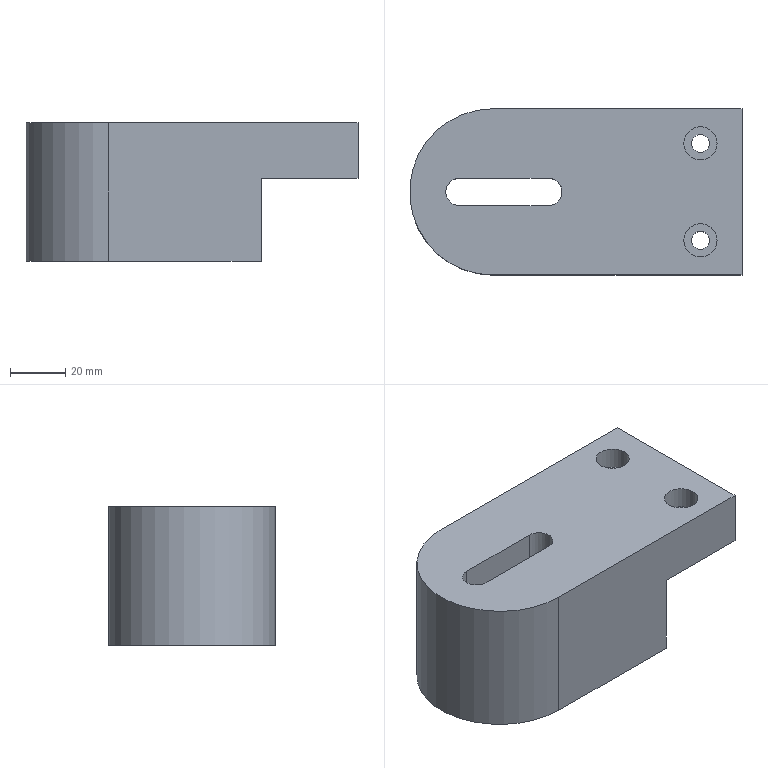Part | NX | 1 solid | 21 faces | box 120 x 60 x 50 mm | volume 252472 mm3 | plane 12 | cylinder 9 | commonest cylinder face diameters 12 x3 6.5 x2 10 x2 5 x1 60 x1
STEP:
#1=CARTESIAN_POINT('',(25.,-30.,-25.));
#2=VERTEX_POINT('',#1);
#3=CARTESIAN_POINT('',(25.,30.,-25.));
#4=VERTEX_POINT('',#3);
#5=CARTESIAN_POINT('',(25.,-30.,-25.));
#6=DIRECTION('',(0.,1.,0.));
#7=VECTOR('',#6,1.);
#8=LINE('',#5,#7);
#9=EDGE_CURVE('',#2,#4,#8,.T.);
#10=ORIENTED_EDGE('',*,*,#9,.F.);
#11=CARTESIAN_POINT('',(-30.,-30.,-25.));
#12=VERTEX_POINT('',#11);
#13=CARTESIAN_POINT('',(-30.,-30.,-25.));
#14=DIRECTION('',(1.,0.,0.));
#15=VECTOR('',#14,1.);
#16=LINE('',#13,#15);
#17=EDGE_CURVE('',#12,#2,#16,.T.);
#18=ORIENTED_EDGE('',*,*,#17,.F.);
#19=CARTESIAN_POINT('',(-30.,30.,-25.));
#20=VERTEX_POINT('',#19);
#21=CARTESIAN_POINT('',(-30.,0.,-25.));
#22=DIRECTION('',(0.,0.,1.));
#23=DIRECTION('',(0.,1.,0.));
#24=AXIS2_PLACEMENT_3D('',#21,#22,#23);
#25=CIRCLE('',#24,30.);
#26=EDGE_CURVE('',#20,#12,#25,.T.);
#27=ORIENTED_EDGE('',*,*,#26,.F.);
#28=CARTESIAN_POINT('',(25.,30.,-25.));
#29=DIRECTION('',(-1.,0.,0.));
#30=VECTOR('',#29,1.);
#31=LINE('',#28,#30);
#32=EDGE_CURVE('',#4,#20,#31,.T.);
#33=ORIENTED_EDGE('',*,*,#32,.F.);
#34=EDGE_LOOP('',(#10,#18,#27,#33));
#35=FACE_BOUND('',#34,.T.);
#36=CARTESIAN_POINT('',(-42.,5.,-25.));
#37=VERTEX_POINT('',#36);
#38=CARTESIAN_POINT('',(-42.,-5.,-25.));
#39=VERTEX_POINT('',#38);
#40=CARTESIAN_POINT('',(-42.,0.,-25.));
#41=DIRECTION('',(0.,0.,1.));
#42=DIRECTION('',(0.,1.,0.));
#43=AXIS2_PLACEMENT_3D('',#40,#41,#42);
#44=CIRCLE('',#43,5.);
#45=EDGE_CURVE('',#37,#39,#44,.T.);
#46=ORIENTED_EDGE('',*,*,#45,.T.);
#47=CARTESIAN_POINT('',(-10.,-5.,-25.));
#48=VERTEX_POINT('',#47);
#49=CARTESIAN_POINT('',(-42.,-5.,-25.));
#50=DIRECTION('',(1.,0.,0.));
#51=VECTOR('',#50,1.);
#52=LINE('',#49,#51);
#53=EDGE_CURVE('',#39,#48,#52,.T.);
#54=ORIENTED_EDGE('',*,*,#53,.T.);
#55=CARTESIAN_POINT('',(-10.,5.,-25.));
#56=VERTEX_POINT('',#55);
#57=CARTESIAN_POINT('',(-10.,0.,-25.));
#58=DIRECTION('',(0.,0.,1.));
#59=DIRECTION('',(0.,-1.,0.));
#60=AXIS2_PLACEMENT_3D('',#57,#58,#59);
#61=CIRCLE('',#60,5.);
#62=EDGE_CURVE('',#48,#56,#61,.T.);
#63=ORIENTED_EDGE('',*,*,#62,.T.);
#64=CARTESIAN_POINT('',(-10.,5.,-25.));
#65=DIRECTION('',(-1.,0.,0.));
#66=VECTOR('',#65,1.);
#67=LINE('',#64,#66);
#68=EDGE_CURVE('',#56,#37,#67,.T.);
#69=ORIENTED_EDGE('',*,*,#68,.T.);
#70=EDGE_LOOP('',(#46,#54,#63,#69));
#71=FACE_BOUND('',#70,.T.);
#72=CARTESIAN_POINT('',(0.,0.,-25.));
#73=DIRECTION('',(0.,0.,1.));
#74=DIRECTION('',(1.,0.,0.));
#75=AXIS2_PLACEMENT_3D('',#72,#73,#74);
#76=PLANE('',#75);
#77=ADVANCED_FACE('',(#35,#71),#76,.F.);
#78=CARTESIAN_POINT('',(-30.,-30.,25.));
#79=VERTEX_POINT('',#78);
#80=CARTESIAN_POINT('',(-30.,30.,25.));
#81=VERTEX_POINT('',#80);
#82=CARTESIAN_POINT('',(-30.,0.,25.));
#83=DIRECTION('',(0.,0.,-1.));
#84=DIRECTION('',(0.,-1.,0.));
#85=AXIS2_PLACEMENT_3D('',#82,#83,#84);
#86=CIRCLE('',#85,30.);
#87=EDGE_CURVE('',#79,#81,#86,.T.);
#88=ORIENTED_EDGE('',*,*,#87,.F.);
#89=CARTESIAN_POINT('',(60.,-30.,25.));
#90=VERTEX_POINT('',#89);
#91=CARTESIAN_POINT('',(-30.,-30.,25.));
#92=DIRECTION('',(1.,0.,0.));
#93=VECTOR('',#92,1.);
#94=LINE('',#91,#93);
#95=EDGE_CURVE('',#79,#90,#94,.T.);
#96=ORIENTED_EDGE('',*,*,#95,.T.);
#97=CARTESIAN_POINT('',(60.,30.,25.));
#98=VERTEX_POINT('',#97);
#99=CARTESIAN_POINT('',(60.,-30.,25.));
#100=DIRECTION('',(0.,1.,0.));
#101=VECTOR('',#100,1.);
#102=LINE('',#99,#101);
#103=EDGE_CURVE('',#90,#98,#102,.T.);
#104=ORIENTED_EDGE('',*,*,#103,.T.);
#105=CARTESIAN_POINT('',(60.,30.,25.));
#106=DIRECTION('',(-1.,0.,0.));
#107=VECTOR('',#106,1.);
#108=LINE('',#105,#107);
#109=EDGE_CURVE('',#98,#81,#108,.T.);
#110=ORIENTED_EDGE('',*,*,#109,.T.);
#111=EDGE_LOOP('',(#88,#96,#104,#110));
#112=FACE_BOUND('',#111,.T.);
#113=CARTESIAN_POINT('',(-42.,5.,25.));
#114=VERTEX_POINT('',#113);
#115=CARTESIAN_POINT('',(-42.,-5.,25.));
#116=VERTEX_POINT('',#115);
#117=CARTESIAN_POINT('',(-42.,0.,25.));
#118=DIRECTION('',(0.,0.,1.));
#119=DIRECTION('',(0.,1.,0.));
#120=AXIS2_PLACEMENT_3D('',#117,#118,#119);
#121=CIRCLE('',#120,5.);
#122=EDGE_CURVE('',#114,#116,#121,.T.);
#123=ORIENTED_EDGE('',*,*,#122,.F.);
#124=CARTESIAN_POINT('',(-10.,5.,25.));
#125=VERTEX_POINT('',#124);
#126=CARTESIAN_POINT('',(-10.,5.,25.));
#127=DIRECTION('',(-1.,0.,0.));
#128=VECTOR('',#127,1.);
#129=LINE('',#126,#128);
#130=EDGE_CURVE('',#125,#114,#129,.T.);
#131=ORIENTED_EDGE('',*,*,#130,.F.);
#132=CARTESIAN_POINT('',(-10.,-5.,25.));
#133=VERTEX_POINT('',#132);
#134=CARTESIAN_POINT('',(-10.,0.,25.));
#135=DIRECTION('',(0.,0.,1.));
#136=DIRECTION('',(0.,-1.,0.));
#137=AXIS2_PLACEMENT_3D('',#134,#135,#136);
#138=CIRCLE('',#137,5.);
#139=EDGE_CURVE('',#133,#125,#138,.T.);
#140=ORIENTED_EDGE('',*,*,#139,.F.);
#141=CARTESIAN_POINT('',(-42.,-5.,25.));
#142=DIRECTION('',(1.,0.,0.));
#143=VECTOR('',#142,1.);
#144=LINE('',#141,#143);
#145=EDGE_CURVE('',#116,#133,#144,.T.);
#146=ORIENTED_EDGE('',*,*,#145,.F.);
#147=EDGE_LOOP('',(#123,#131,#140,#146));
#148=FACE_BOUND('',#147,.T.);
#149=CARTESIAN_POINT('',(51.,17.5,25.));
#150=VERTEX_POINT('',#149);
#151=CARTESIAN_POINT('',(45.,17.5,25.));
#152=DIRECTION('',(0.,0.,1.));
#153=DIRECTION('',(1.,0.,0.));
#154=AXIS2_PLACEMENT_3D('',#151,#152,#153);
#155=CIRCLE('',#154,6.);
#156=EDGE_CURVE('',#150,#150,#155,.T.);
#157=ORIENTED_EDGE('',*,*,#156,.F.);
#158=EDGE_LOOP('',(#157));
#159=FACE_BOUND('',#158,.T.);
#160=CARTESIAN_POINT('',(51.,-17.5,25.));
#161=VERTEX_POINT('',#160);
#162=CARTESIAN_POINT('',(45.,-17.5,25.));
#163=DIRECTION('',(0.,0.,1.));
#164=DIRECTION('',(1.,0.,0.));
#165=AXIS2_PLACEMENT_3D('',#162,#163,#164);
#166=CIRCLE('',#165,6.);
#167=EDGE_CURVE('',#161,#161,#166,.T.);
#168=ORIENTED_EDGE('',*,*,#167,.F.);
#169=EDGE_LOOP('',(#168));
#170=FACE_BOUND('',#169,.T.);
#171=CARTESIAN_POINT('',(0.,0.,25.));
#172=DIRECTION('',(0.,0.,1.));
#173=DIRECTION('',(1.,0.,0.));
#174=AXIS2_PLACEMENT_3D('',#171,#172,#173);
#175=PLANE('',#174);
#176=ADVANCED_FACE('',(#112,#148,#159,#170),#175,.T.);
#177=CARTESIAN_POINT('',(60.,-30.,5.));
#178=VERTEX_POINT('',#177);
#179=CARTESIAN_POINT('',(25.,-30.,5.));
#180=VERTEX_POINT('',#179);
#181=CARTESIAN_POINT('',(60.,-30.,5.));
#182=DIRECTION('',(-1.,0.,0.));
#183=VECTOR('',#182,1.);
#184=LINE('',#181,#183);
#185=EDGE_CURVE('',#178,#180,#184,.T.);
#186=ORIENTED_EDGE('',*,*,#185,.F.);
#187=CARTESIAN_POINT('',(60.,-30.,5.));
#188=DIRECTION('',(0.,0.,1.));
#189=VECTOR('',#188,1.);
#190=LINE('',#187,#189);
#191=EDGE_CURVE('',#178,#90,#190,.T.);
#192=ORIENTED_EDGE('',*,*,#191,.T.);
#193=ORIENTED_EDGE('',*,*,#95,.F.);
#194=CARTESIAN_POINT('',(-30.,-30.,25.));
#195=DIRECTION('',(0.,0.,-1.));
#196=VECTOR('',#195,1.);
#197=LINE('',#194,#196);
#198=EDGE_CURVE('',#79,#12,#197,.T.);
#199=ORIENTED_EDGE('',*,*,#198,.T.);
#200=ORIENTED_EDGE('',*,*,#17,.T.);
#201=CARTESIAN_POINT('',(25.,-30.,-25.));
#202=DIRECTION('',(0.,0.,1.));
#203=VECTOR('',#202,1.);
#204=LINE('',#201,#203);
#205=EDGE_CURVE('',#2,#180,#204,.T.);
#206=ORIENTED_EDGE('',*,*,#205,.T.);
#207=EDGE_LOOP('',(#186,#192,#193,#199,#200,#206));
#208=FACE_OUTER_BOUND('',#207,.T.);
#209=CARTESIAN_POINT('',(-60.,-30.,-25.));
#210=DIRECTION('',(0.,-1.,0.));
#211=DIRECTION('',(0.,0.,-1.));
#212=AXIS2_PLACEMENT_3D('',#209,#210,#211);
#213=PLANE('',#212);
#214=ADVANCED_FACE('',(#208),#213,.T.);
#215=CARTESIAN_POINT('',(60.,30.,5.));
#216=VERTEX_POINT('',#215);
#217=CARTESIAN_POINT('',(60.,-30.,5.));
#218=DIRECTION('',(0.,1.,0.));
#219=VECTOR('',#218,1.);
#220=LINE('',#217,#219);
#221=EDGE_CURVE('',#178,#216,#220,.T.);
#222=ORIENTED_EDGE('',*,*,#221,.T.);
#223=CARTESIAN_POINT('',(60.,30.,5.));
#224=DIRECTION('',(0.,0.,1.));
#225=VECTOR('',#224,1.);
#226=LINE('',#223,#225);
#227=EDGE_CURVE('',#216,#98,#226,.T.);
#228=ORIENTED_EDGE('',*,*,#227,.T.);
#229=ORIENTED_EDGE('',*,*,#103,.F.);
#230=ORIENTED_EDGE('',*,*,#191,.F.);
#231=EDGE_LOOP('',(#222,#228,#229,#230));
#232=FACE_BOUND('',#231,.T.);
#233=CARTESIAN_POINT('',(60.,0.,9.));
#234=VERTEX_POINT('',#233);
#235=CARTESIAN_POINT('',(60.,0.,15.));
#236=DIRECTION('',(1.,0.,0.));
#237=DIRECTION('',(0.,0.,-1.));
#238=AXIS2_PLACEMENT_3D('',#235,#236,#237);
#239=CIRCLE('',#238,6.);
#240=EDGE_CURVE('',#234,#234,#239,.T.);
#241=ORIENTED_EDGE('',*,*,#240,.F.);
#242=EDGE_LOOP('',(#241));
#243=FACE_BOUND('',#242,.T.);
#244=CARTESIAN_POINT('',(60.,-30.,-25.));
#245=DIRECTION('',(1.,0.,0.));
#246=DIRECTION('',(0.,0.,-1.));
#247=AXIS2_PLACEMENT_3D('',#244,#245,#246);
#248=PLANE('',#247);
#249=ADVANCED_FACE('',(#232,#243),#248,.T.);
#250=CARTESIAN_POINT('',(25.,30.,5.));
#251=VERTEX_POINT('',#250);
#252=CARTESIAN_POINT('',(60.,30.,5.));
#253=DIRECTION('',(-1.,0.,0.));
#254=VECTOR('',#253,1.);
#255=LINE('',#252,#254);
#256=EDGE_CURVE('',#216,#251,#255,.T.);
#257=ORIENTED_EDGE('',*,*,#256,.T.);
#258=CARTESIAN_POINT('',(25.,30.,-25.));
#259=DIRECTION('',(0.,0.,1.));
#260=VECTOR('',#259,1.);
#261=LINE('',#258,#260);
#262=EDGE_CURVE('',#4,#251,#261,.T.);
#263=ORIENTED_EDGE('',*,*,#262,.F.);
#264=ORIENTED_EDGE('',*,*,#32,.T.);
#265=CARTESIAN_POINT('',(-30.,30.,25.));
#266=DIRECTION('',(0.,0.,-1.));
#267=VECTOR('',#266,1.);
#268=LINE('',#265,#267);
#269=EDGE_CURVE('',#81,#20,#268,.T.);
#270=ORIENTED_EDGE('',*,*,#269,.F.);
#271=ORIENTED_EDGE('',*,*,#109,.F.);
#272=ORIENTED_EDGE('',*,*,#227,.F.);
#273=EDGE_LOOP('',(#257,#263,#264,#270,#271,#272));
#274=FACE_OUTER_BOUND('',#273,.T.);
#275=CARTESIAN_POINT('',(60.,30.,-25.));
#276=DIRECTION('',(0.,1.,0.));
#277=DIRECTION('',(0.,0.,1.));
#278=AXIS2_PLACEMENT_3D('',#275,#276,#277);
#279=PLANE('',#278);
#280=ADVANCED_FACE('',(#274),#279,.T.);
#281=ORIENTED_EDGE('',*,*,#87,.T.);
#282=ORIENTED_EDGE('',*,*,#269,.T.);
#283=ORIENTED_EDGE('',*,*,#26,.T.);
#284=ORIENTED_EDGE('',*,*,#198,.F.);
#285=EDGE_LOOP('',(#281,#282,#283,#284));
#286=FACE_OUTER_BOUND('',#285,.T.);
#287=CARTESIAN_POINT('',(-30.,0.,25.231));
#288=DIRECTION('',(0.,0.,-1.));
#289=DIRECTION('',(-1.,0.,0.));
#290=AXIS2_PLACEMENT_3D('',#287,#288,#289);
#291=CYLINDRICAL_SURFACE('',#290,30.);
#292=ADVANCED_FACE('',(#286),#291,.T.);
#293=ORIENTED_EDGE('',*,*,#185,.T.);
#294=CARTESIAN_POINT('',(25.,-30.,5.));
#295=DIRECTION('',(0.,1.,0.));
#296=VECTOR('',#295,1.);
#297=LINE('',#294,#296);
#298=EDGE_CURVE('',#180,#251,#297,.T.);
#299=ORIENTED_EDGE('',*,*,#298,.T.);
#300=ORIENTED_EDGE('',*,*,#256,.F.);
#301=ORIENTED_EDGE('',*,*,#221,.F.);
#302=EDGE_LOOP('',(#293,#299,#300,#301));
#303=FACE_BOUND('',#302,.T.);
#304=CARTESIAN_POINT('',(48.25,17.5,5.));
#305=VERTEX_POINT('',#304);
#306=CARTESIAN_POINT('',(45.,17.5,5.));
#307=DIRECTION('',(0.,0.,1.));
#308=DIRECTION('',(1.,0.,0.));
#309=AXIS2_PLACEMENT_3D('',#306,#307,#308);
#310=CIRCLE('',#309,3.25);
#311=EDGE_CURVE('',#305,#305,#310,.T.);
#312=ORIENTED_EDGE('',*,*,#311,.T.);
#313=EDGE_LOOP('',(#312));
#314=FACE_BOUND('',#313,.T.);
#315=CARTESIAN_POINT('',(48.25,-17.5,5.));
#316=VERTEX_POINT('',#315);
#317=CARTESIAN_POINT('',(45.,-17.5,5.));
#318=DIRECTION('',(0.,0.,1.));
#319=DIRECTION('',(1.,0.,0.));
#320=AXIS2_PLACEMENT_3D('',#317,#318,#319);
#321=CIRCLE('',#320,3.25);
#322=EDGE_CURVE('',#316,#316,#321,.T.);
#323=ORIENTED_EDGE('',*,*,#322,.T.);
#324=EDGE_LOOP('',(#323));
#325=FACE_BOUND('',#324,.T.);
#326=CARTESIAN_POINT('',(0.,0.,5.));
#327=DIRECTION('',(0.,0.,-1.));
#328=DIRECTION('',(-1.,0.,0.));
#329=AXIS2_PLACEMENT_3D('',#326,#327,#328);
#330=PLANE('',#329);
#331=ADVANCED_FACE('',(#303,#314,#325),#330,.T.);
#332=ORIENTED_EDGE('',*,*,#9,.T.);
#333=ORIENTED_EDGE('',*,*,#262,.T.);
#334=ORIENTED_EDGE('',*,*,#298,.F.);
#335=ORIENTED_EDGE('',*,*,#205,.F.);
#336=EDGE_LOOP('',(#332,#333,#334,#335));
#337=FACE_OUTER_BOUND('',#336,.T.);
#338=CARTESIAN_POINT('',(25.,-30.,-25.));
#339=DIRECTION('',(-1.,0.,0.));
#340=DIRECTION('',(0.,0.,1.));
#341=AXIS2_PLACEMENT_3D('',#338,#339,#340);
#342=PLANE('',#341);
#343=ADVANCED_FACE('',(#337),#342,.F.);
#344=ORIENTED_EDGE('',*,*,#45,.F.);
#345=CARTESIAN_POINT('',(-42.,5.,25.));
#346=DIRECTION('',(0.,0.,-1.));
#347=VECTOR('',#346,1.);
#348=LINE('',#345,#347);
#349=EDGE_CURVE('',#114,#37,#348,.T.);
#350=ORIENTED_EDGE('',*,*,#349,.F.);
#351=ORIENTED_EDGE('',*,*,#122,.T.);
#352=CARTESIAN_POINT('',(-42.,-5.,25.));
#353=DIRECTION('',(0.,0.,-1.));
#354=VECTOR('',#353,1.);
#355=LINE('',#352,#354);
#356=EDGE_CURVE('',#116,#39,#355,.T.);
#357=ORIENTED_EDGE('',*,*,#356,.T.);
#358=EDGE_LOOP('',(#344,#350,#351,#357));
#359=FACE_OUTER_BOUND('',#358,.T.);
#360=CARTESIAN_POINT('',(-42.,0.,25.));
#361=DIRECTION('',(0.,0.,1.));
#362=DIRECTION('',(1.,0.,0.));
#363=AXIS2_PLACEMENT_3D('',#360,#361,#362);
#364=CYLINDRICAL_SURFACE('',#363,5.);
#365=ADVANCED_FACE('',(#359),#364,.F.);
#366=ORIENTED_EDGE('',*,*,#53,.F.);
#367=ORIENTED_EDGE('',*,*,#356,.F.);
#368=ORIENTED_EDGE('',*,*,#145,.T.);
#369=CARTESIAN_POINT('',(-10.,-5.,25.));
#370=DIRECTION('',(0.,0.,-1.));
#371=VECTOR('',#370,1.);
#372=LINE('',#369,#371);
#373=EDGE_CURVE('',#133,#48,#372,.T.);
#374=ORIENTED_EDGE('',*,*,#373,.T.);
#375=EDGE_LOOP('',(#366,#367,#368,#374));
#376=FACE_OUTER_BOUND('',#375,.T.);
#377=CARTESIAN_POINT('',(-42.,-5.,25.));
#378=DIRECTION('',(0.,-1.,0.));
#379=DIRECTION('',(0.,0.,-1.));
#380=AXIS2_PLACEMENT_3D('',#377,#378,#379);
#381=PLANE('',#380);
#382=ADVANCED_FACE('',(#376),#381,.F.);
#383=ORIENTED_EDGE('',*,*,#62,.F.);
#384=ORIENTED_EDGE('',*,*,#373,.F.);
#385=ORIENTED_EDGE('',*,*,#139,.T.);
#386=CARTESIAN_POINT('',(-10.,5.,25.));
#387=DIRECTION('',(0.,0.,-1.));
#388=VECTOR('',#387,1.);
#389=LINE('',#386,#388);
#390=EDGE_CURVE('',#125,#56,#389,.T.);
#391=ORIENTED_EDGE('',*,*,#390,.T.);
#392=EDGE_LOOP('',(#383,#384,#385,#391));
#393=FACE_BOUND('',#392,.T.);
#394=CARTESIAN_POINT('',(-5.,-0.000000402,12.5));
#395=VERTEX_POINT('',#394);
#396=CARTESIAN_POINT('',(-5.,-0.000000402,12.5));
#397=CARTESIAN_POINT('',(-5.,0.262,12.5));
#398=CARTESIAN_POINT('',(-5.022,0.5275,12.543));
#399=CARTESIAN_POINT('',(-5.06,0.7739,12.623));
#400=CARTESIAN_POINT('',(-5.099,1.02,12.703));
#401=CARTESIAN_POINT('',(-5.155,1.253,12.822));
#402=CARTESIAN_POINT('',(-5.218,1.459,12.97));
#403=CARTESIAN_POINT('',(-5.284,1.678,13.127));
#404=CARTESIAN_POINT('',(-5.36,1.871,13.321));
#405=CARTESIAN_POINT('',(-5.43,2.028,13.538));
#406=CARTESIAN_POINT('',(-5.505,2.197,13.773));
#407=CARTESIAN_POINT('',(-5.574,2.328,14.043));
#408=CARTESIAN_POINT('',(-5.618,2.408,14.327));
#409=CARTESIAN_POINT('',(-5.659,2.482,14.594));
#410=CARTESIAN_POINT('',(-5.677,2.513,14.883));
#411=CARTESIAN_POINT('',(-5.667,2.495,15.162));
#412=CARTESIAN_POINT('',(-5.658,2.479,15.408));
#413=CARTESIAN_POINT('',(-5.626,2.425,15.654));
#414=CARTESIAN_POINT('',(-5.581,2.34,15.881));
#415=CARTESIAN_POINT('',(-5.535,2.252,16.114));
#416=CARTESIAN_POINT('',(-5.473,2.129,16.333));
#417=CARTESIAN_POINT('',(-5.409,1.98,16.527));
#418=CARTESIAN_POINT('',(-5.336,1.811,16.745));
#419=CARTESIAN_POINT('',(-5.258,1.605,16.937));
#420=CARTESIAN_POINT('',(-5.192,1.373,17.089));
#421=CARTESIAN_POINT('',(-5.123,1.131,17.248));
#422=CARTESIAN_POINT('',(-5.065,0.8533,17.368));
#423=CARTESIAN_POINT('',(-5.032,0.5649,17.435));
#424=CARTESIAN_POINT('',(-5.002,0.3005,17.497));
#425=CARTESIAN_POINT('',(-4.993,0.01906,17.515));
#426=CARTESIAN_POINT('',(-5.006,-0.2523,17.487));
#427=CARTESIAN_POINT('',(-5.019,-0.5027,17.462));
#428=CARTESIAN_POINT('',(-5.051,-0.7513,17.397));
#429=CARTESIAN_POINT('',(-5.097,-0.9794,17.3));
#430=CARTESIAN_POINT('',(-5.144,-1.214,17.2));
#431=CARTESIAN_POINT('',(-5.206,-1.433,17.064));
#432=CARTESIAN_POINT('',(-5.271,-1.624,16.901));
#433=CARTESIAN_POINT('',(-5.343,-1.834,16.721));
#434=CARTESIAN_POINT('',(-5.421,-2.015,16.506));
#435=CARTESIAN_POINT('',(-5.488,-2.155,16.267));
#436=CARTESIAN_POINT('',(-5.559,-2.302,16.017));
#437=CARTESIAN_POINT('',(-5.618,-2.409,15.733));
#438=CARTESIAN_POINT('',(-5.648,-2.461,15.441));
#439=CARTESIAN_POINT('',(-5.674,-2.508,15.177));
#440=CARTESIAN_POINT('',(-5.677,-2.512,14.898));
#441=CARTESIAN_POINT('',(-5.654,-2.473,14.632));
#442=CARTESIAN_POINT('',(-5.634,-2.437,14.391));
#443=CARTESIAN_POINT('',(-5.593,-2.365,14.155));
#444=CARTESIAN_POINT('',(-5.542,-2.264,13.939));
#445=CARTESIAN_POINT('',(-5.487,-2.156,13.708));
#446=CARTESIAN_POINT('',(-5.419,-2.012,13.495));
#447=CARTESIAN_POINT('',(-5.351,-1.841,13.309));
#448=CARTESIAN_POINT('',(-5.276,-1.65,13.101));
#449=CARTESIAN_POINT('',(-5.199,-1.421,12.923));
#450=CARTESIAN_POINT('',(-5.138,-1.168,12.79));
#451=CARTESIAN_POINT('',(-5.077,-0.9137,12.655));
#452=CARTESIAN_POINT('',(-5.031,-0.6278,12.562));
#453=CARTESIAN_POINT('',(-5.011,-0.3373,12.523));
#454=CARTESIAN_POINT('',(-5.004,-0.2258,12.508));
#455=CARTESIAN_POINT('',(-5.,-0.1128,12.5));
#456=CARTESIAN_POINT('',(-5.,-0.000000402,12.5));
#457=B_SPLINE_CURVE_WITH_KNOTS('',3,(#396,#397,#398,#399,#400,#401,#402,#403,#404,#405,#406,#407,#408,#409,#410,#411,#412,#413,#414,#415,#416,#417,#418,#419,#420,#421,#422,#423,#424,#425,#426,#427,#428,#429,#430,#431,#432,#433,#434,#435,#436,#437,#438,#439,#440,#441,#442,#443,#444,#445,#446,#447,#448,#449,#450,#451,#452,#453,#454,#455,#456),.UNSPECIFIED.,.T.,.F.,(1,3,3,3,3,3,3,3,3,3,3,3,3,3,3,3,3,3,3,3,3,3,1),(-0.02098,0.,0.04946,0.09871,0.151,0.2074,0.2605,0.307,0.3546,0.4083,0.4646,0.5162,0.5637,0.6125,0.6662,0.7226,0.7735,0.8194,0.8684,0.9235,0.979,1.,1.049),.UNSPECIFIED.);
#458=EDGE_CURVE('',#395,#395,#457,.T.);
#459=ORIENTED_EDGE('',*,*,#458,.T.);
#460=EDGE_LOOP('',(#459));
#461=FACE_BOUND('',#460,.T.);
#462=CARTESIAN_POINT('',(-10.,0.,25.));
#463=DIRECTION('',(0.,0.,1.));
#464=DIRECTION('',(1.,0.,0.));
#465=AXIS2_PLACEMENT_3D('',#462,#463,#464);
#466=CYLINDRICAL_SURFACE('',#465,5.);
#467=ADVANCED_FACE('',(#393,#461),#466,.F.);
#468=ORIENTED_EDGE('',*,*,#68,.F.);
#469=ORIENTED_EDGE('',*,*,#390,.F.);
#470=ORIENTED_EDGE('',*,*,#130,.T.);
#471=ORIENTED_EDGE('',*,*,#349,.T.);
#472=EDGE_LOOP('',(#468,#469,#470,#471));
#473=FACE_OUTER_BOUND('',#472,.T.);
#474=CARTESIAN_POINT('',(-10.,5.,25.));
#475=DIRECTION('',(0.,1.,0.));
#476=DIRECTION('',(0.,0.,1.));
#477=AXIS2_PLACEMENT_3D('',#474,#475,#476);
#478=PLANE('',#477);
#479=ADVANCED_FACE('',(#473),#478,.F.);
#480=CARTESIAN_POINT('',(45.,0.,12.5));
#481=VERTEX_POINT('',#480);
#482=CARTESIAN_POINT('',(45.,0.,15.));
#483=DIRECTION('',(1.,0.,0.));
#484=DIRECTION('',(0.,0.,-1.));
#485=AXIS2_PLACEMENT_3D('',#482,#483,#484);
#486=CIRCLE('',#485,2.5);
#487=EDGE_CURVE('',#481,#481,#486,.T.);
#488=ORIENTED_EDGE('',*,*,#487,.T.);
#489=EDGE_LOOP('',(#488));
#490=FACE_BOUND('',#489,.T.);
#491=ORIENTED_EDGE('',*,*,#458,.F.);
#492=EDGE_LOOP('',(#491));
#493=FACE_BOUND('',#492,.T.);
#494=CARTESIAN_POINT('',(60.,0.,15.));
#495=DIRECTION('',(1.,0.,0.));
#496=DIRECTION('',(0.,0.,-1.));
#497=AXIS2_PLACEMENT_3D('',#494,#495,#496);
#498=CYLINDRICAL_SURFACE('',#497,2.5);
#499=ADVANCED_FACE('',(#490,#493),#498,.F.);
#500=CARTESIAN_POINT('',(45.,0.,9.));
#501=VERTEX_POINT('',#500);
#502=CARTESIAN_POINT('',(45.,0.,15.));
#503=DIRECTION('',(1.,0.,0.));
#504=DIRECTION('',(0.,0.,-1.));
#505=AXIS2_PLACEMENT_3D('',#502,#503,#504);
#506=CIRCLE('',#505,6.);
#507=EDGE_CURVE('',#501,#501,#506,.T.);
#508=ORIENTED_EDGE('',*,*,#507,.T.);
#509=EDGE_LOOP('',(#508));
#510=FACE_BOUND('',#509,.T.);
#511=ORIENTED_EDGE('',*,*,#487,.F.);
#512=EDGE_LOOP('',(#511));
#513=FACE_BOUND('',#512,.T.);
#514=CARTESIAN_POINT('',(45.,0.,-25.));
#515=DIRECTION('',(1.,0.,0.));
#516=DIRECTION('',(0.,0.,-1.));
#517=AXIS2_PLACEMENT_3D('',#514,#515,#516);
#518=PLANE('',#517);
#519=ADVANCED_FACE('',(#510,#513),#518,.T.);
#520=ORIENTED_EDGE('',*,*,#240,.T.);
#521=EDGE_LOOP('',(#520));
#522=FACE_BOUND('',#521,.T.);
#523=ORIENTED_EDGE('',*,*,#507,.F.);
#524=EDGE_LOOP('',(#523));
#525=FACE_BOUND('',#524,.T.);
#526=CARTESIAN_POINT('',(60.,0.,15.));
#527=DIRECTION('',(1.,0.,0.));
#528=DIRECTION('',(0.,0.,-1.));
#529=AXIS2_PLACEMENT_3D('',#526,#527,#528);
#530=CYLINDRICAL_SURFACE('',#529,6.);
#531=ADVANCED_FACE('',(#522,#525),#530,.F.);
#532=CARTESIAN_POINT('',(48.25,17.5,17.));
#533=VERTEX_POINT('',#532);
#534=CARTESIAN_POINT('',(45.,17.5,17.));
#535=DIRECTION('',(0.,0.,1.));
#536=DIRECTION('',(1.,0.,0.));
#537=AXIS2_PLACEMENT_3D('',#534,#535,#536);
#538=CIRCLE('',#537,3.25);
#539=EDGE_CURVE('',#533,#533,#538,.T.);
#540=ORIENTED_EDGE('',*,*,#539,.T.);
#541=EDGE_LOOP('',(#540));
#542=FACE_BOUND('',#541,.T.);
#543=ORIENTED_EDGE('',*,*,#311,.F.);
#544=EDGE_LOOP('',(#543));
#545=FACE_BOUND('',#544,.T.);
#546=CARTESIAN_POINT('',(45.,17.5,25.));
#547=DIRECTION('',(0.,0.,1.));
#548=DIRECTION('',(1.,0.,0.));
#549=AXIS2_PLACEMENT_3D('',#546,#547,#548);
#550=CYLINDRICAL_SURFACE('',#549,3.25);
#551=ADVANCED_FACE('',(#542,#545),#550,.F.);
#552=CARTESIAN_POINT('',(48.25,-17.5,17.));
#553=VERTEX_POINT('',#552);
#554=CARTESIAN_POINT('',(45.,-17.5,17.));
#555=DIRECTION('',(0.,0.,1.));
#556=DIRECTION('',(1.,0.,0.));
#557=AXIS2_PLACEMENT_3D('',#554,#555,#556);
#558=CIRCLE('',#557,3.25);
#559=EDGE_CURVE('',#553,#553,#558,.T.);
#560=ORIENTED_EDGE('',*,*,#559,.T.);
#561=EDGE_LOOP('',(#560));
#562=FACE_BOUND('',#561,.T.);
#563=ORIENTED_EDGE('',*,*,#322,.F.);
#564=EDGE_LOOP('',(#563));
#565=FACE_BOUND('',#564,.T.);
#566=CARTESIAN_POINT('',(45.,-17.5,25.));
#567=DIRECTION('',(0.,0.,1.));
#568=DIRECTION('',(1.,0.,0.));
#569=AXIS2_PLACEMENT_3D('',#566,#567,#568);
#570=CYLINDRICAL_SURFACE('',#569,3.25);
#571=ADVANCED_FACE('',(#562,#565),#570,.F.);
#572=CARTESIAN_POINT('',(51.,17.5,17.));
#573=VERTEX_POINT('',#572);
#574=CARTESIAN_POINT('',(45.,17.5,17.));
#575=DIRECTION('',(0.,0.,1.));
#576=DIRECTION('',(1.,0.,0.));
#577=AXIS2_PLACEMENT_3D('',#574,#575,#576);
#578=CIRCLE('',#577,6.);
#579=EDGE_CURVE('',#573,#573,#578,.T.);
#580=ORIENTED_EDGE('',*,*,#579,.T.);
#581=EDGE_LOOP('',(#580));
#582=FACE_BOUND('',#581,.T.);
#583=ORIENTED_EDGE('',*,*,#539,.F.);
#584=EDGE_LOOP('',(#583));
#585=FACE_BOUND('',#584,.T.);
#586=CARTESIAN_POINT('',(0.,0.,17.));
#587=DIRECTION('',(0.,0.,1.));
#588=DIRECTION('',(1.,0.,0.));
#589=AXIS2_PLACEMENT_3D('',#586,#587,#588);
#590=PLANE('',#589);
#591=ADVANCED_FACE('',(#582,#585),#590,.T.);
#592=CARTESIAN_POINT('',(51.,-17.5,17.));
#593=VERTEX_POINT('',#592);
#594=CARTESIAN_POINT('',(45.,-17.5,17.));
#595=DIRECTION('',(0.,0.,1.));
#596=DIRECTION('',(1.,0.,0.));
#597=AXIS2_PLACEMENT_3D('',#594,#595,#596);
#598=CIRCLE('',#597,6.);
#599=EDGE_CURVE('',#593,#593,#598,.T.);
#600=ORIENTED_EDGE('',*,*,#599,.T.);
#601=EDGE_LOOP('',(#600));
#602=FACE_BOUND('',#601,.T.);
#603=ORIENTED_EDGE('',*,*,#559,.F.);
#604=EDGE_LOOP('',(#603));
#605=FACE_BOUND('',#604,.T.);
#606=CARTESIAN_POINT('',(0.,0.,17.));
#607=DIRECTION('',(0.,0.,1.));
#608=DIRECTION('',(1.,0.,0.));
#609=AXIS2_PLACEMENT_3D('',#606,#607,#608);
#610=PLANE('',#609);
#611=ADVANCED_FACE('',(#602,#605),#610,.T.);
#612=ORIENTED_EDGE('',*,*,#156,.T.);
#613=EDGE_LOOP('',(#612));
#614=FACE_BOUND('',#613,.T.);
#615=ORIENTED_EDGE('',*,*,#579,.F.);
#616=EDGE_LOOP('',(#615));
#617=FACE_BOUND('',#616,.T.);
#618=CARTESIAN_POINT('',(45.,17.5,25.));
#619=DIRECTION('',(0.,0.,1.));
#620=DIRECTION('',(1.,0.,0.));
#621=AXIS2_PLACEMENT_3D('',#618,#619,#620);
#622=CYLINDRICAL_SURFACE('',#621,6.);
#623=ADVANCED_FACE('',(#614,#617),#622,.F.);
#624=ORIENTED_EDGE('',*,*,#167,.T.);
#625=EDGE_LOOP('',(#624));
#626=FACE_BOUND('',#625,.T.);
#627=ORIENTED_EDGE('',*,*,#599,.F.);
#628=EDGE_LOOP('',(#627));
#629=FACE_BOUND('',#628,.T.);
#630=CARTESIAN_POINT('',(45.,-17.5,25.));
#631=DIRECTION('',(0.,0.,1.));
#632=DIRECTION('',(1.,0.,0.));
#633=AXIS2_PLACEMENT_3D('',#630,#631,#632);
#634=CYLINDRICAL_SURFACE('',#633,6.);
#635=ADVANCED_FACE('',(#626,#629),#634,.F.);
#636=CLOSED_SHELL('',(#77,#176,#214,#249,#280,#292,#331,#343,#365,#382,#467,#479,#499,#519,#531,#551,#571,#591,#611,#623,#635));
#637=MANIFOLD_SOLID_BREP('',#636);
#638=(LENGTH_UNIT()NAMED_UNIT(*)SI_UNIT(.MILLI.,.METRE.));
#639=UNCERTAINTY_MEASURE_WITH_UNIT(LENGTH_MEASURE(0.0508),#638,'','');
#640=(NAMED_UNIT(*)PLANE_ANGLE_UNIT()SI_UNIT($,.RADIAN.));
#641=PLANE_ANGLE_MEASURE_WITH_UNIT(PLANE_ANGLE_MEASURE(0.01745),#640);
#642=DIMENSIONAL_EXPONENTS(0.,0.,0.,0.,0.,0.,0.);
#643=(CONVERSION_BASED_UNIT('DEGREE',#641)NAMED_UNIT(#642)PLANE_ANGLE_UNIT());
#644=(NAMED_UNIT(*)SI_UNIT($,.STERADIAN.)SOLID_ANGLE_UNIT());
#645=(GEOMETRIC_REPRESENTATION_CONTEXT(3)GLOBAL_UNCERTAINTY_ASSIGNED_CONTEXT((#639))GLOBAL_UNIT_ASSIGNED_CONTEXT((#638,#643,#644))REPRESENTATION_CONTEXT('',''));
#646=ADVANCED_BREP_SHAPE_REPRESENTATION('',(#637),#645);